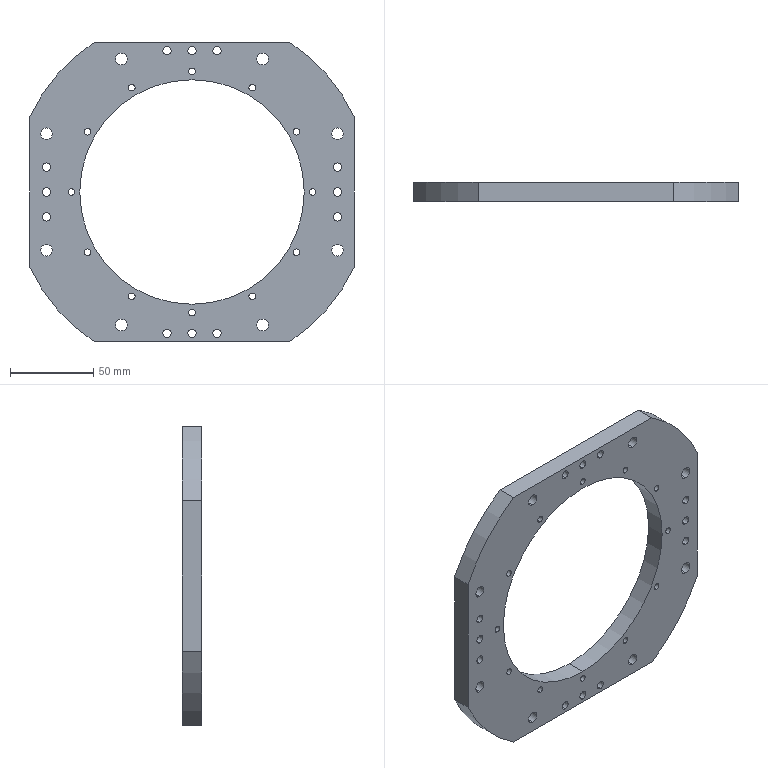Part | STEP file | 2026.6.15-Main Assembly图.sldasm-Part-115 | 1 solid | 76 faces | box 195 x 11.5 x 180 mm | volume 198792 mm3 | cylinder 70 | plane 6 | commonest cylinder face diameters 4 x24 5 x24 7 x16 215 x4 135 x2